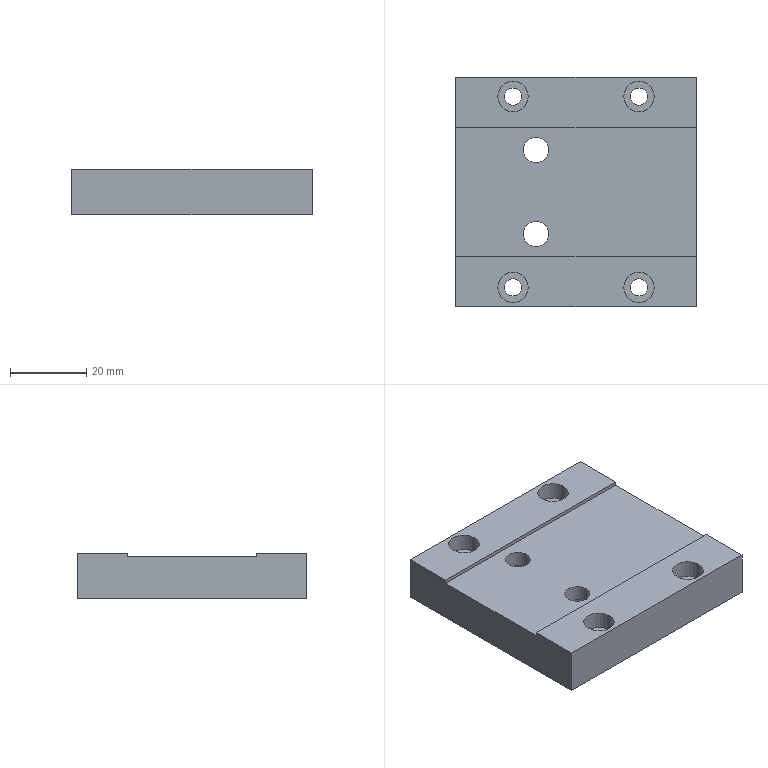Part | STEP file | 2038 Bag feed cylinder mounting plate 12 | 1 solid | 40 faces | box 63 x 60 x 12 mm | volume 40268 mm3 | cylinder 24 | plane 16 | commonest cylinder face diameters 4.5 x8 8 x8 6.6 x4 11 x4